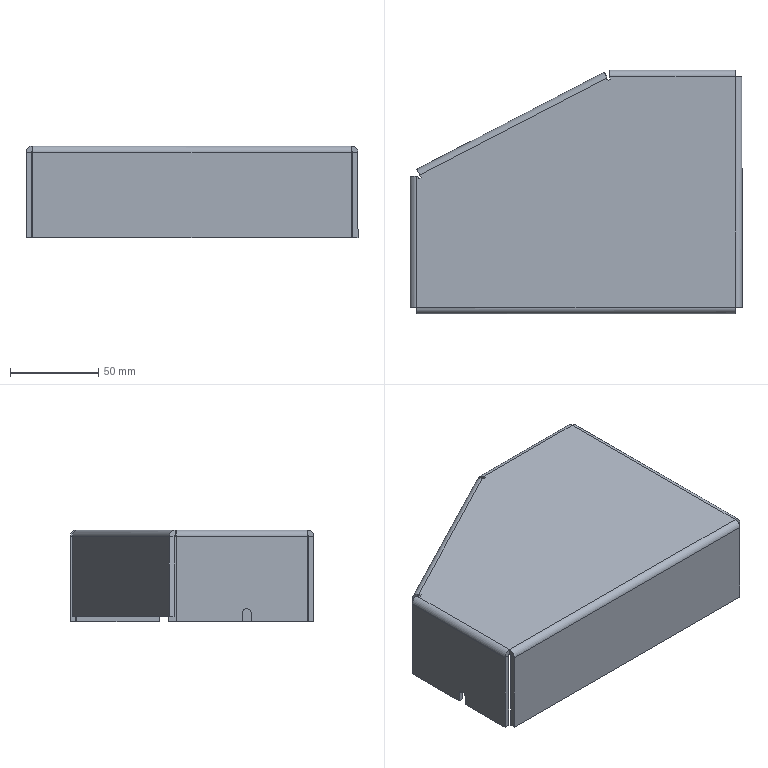Part | SolidWorks | features ICE 3, EdgeFlange 2, FlatPattern 1, SMBaseFlange 1, SheetMetal 1 | 1 solid | 71 faces | box 188 x 138 x 52 mm | volume 149512 mm3 | plane 49 | cylinder 15 | spline 7 | commonest cylinder face diameters 1.473 x5 5 x5 7.473 x5